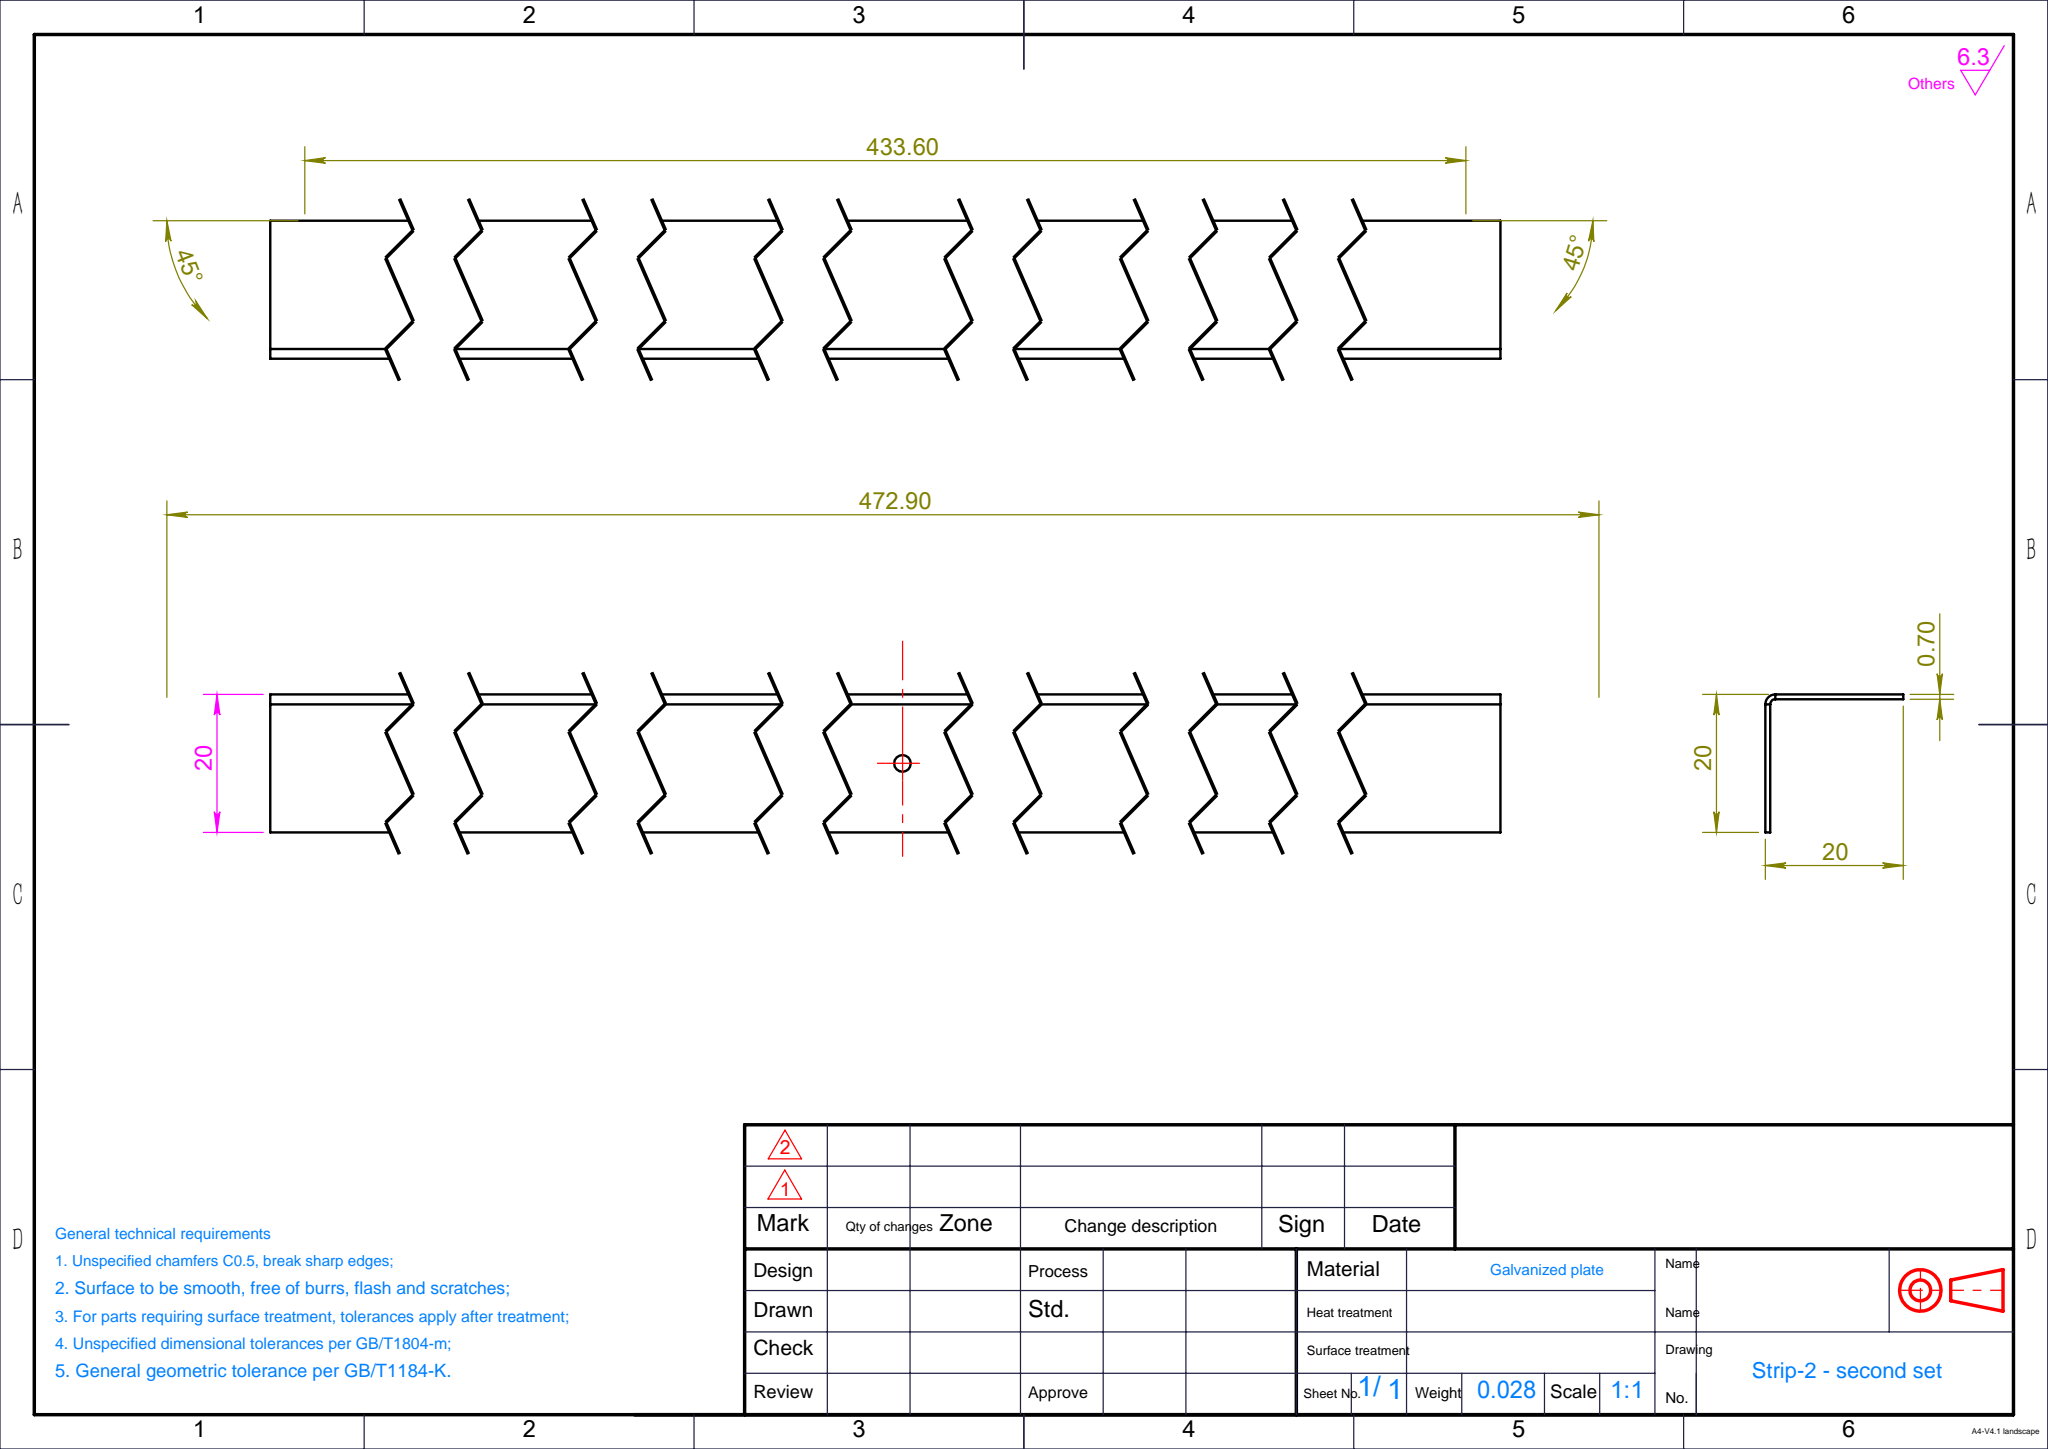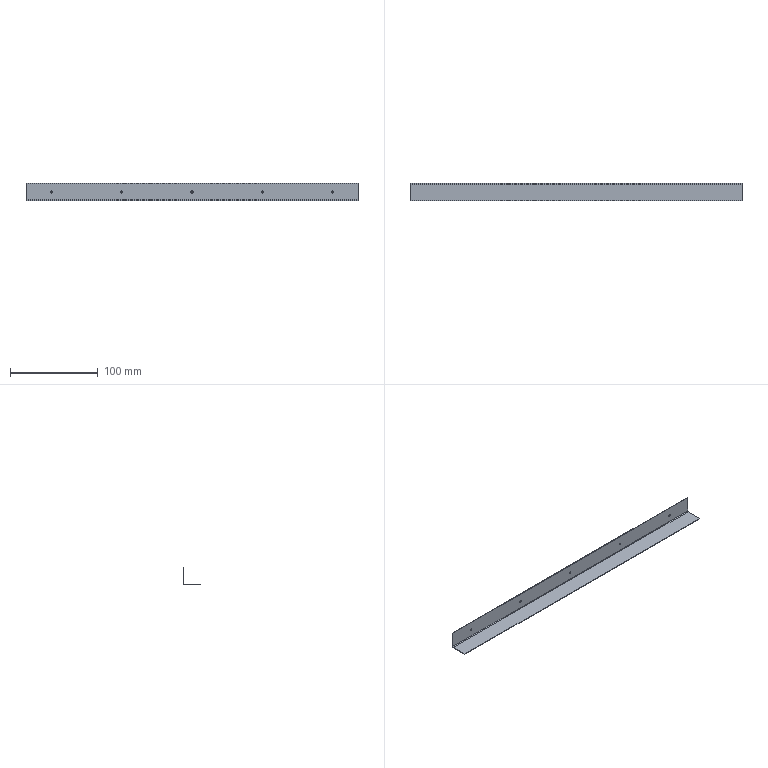Part | SolidWorks | features 3DProfileFeature 1, EdgeFlange 1, FlatPattern 1, HoleWzd 1, LPattern 1, MirrorPattern 1, SMBaseFlange 1, SheetMetal 1 | 1 solid | 24 faces | box 378 x 20 x 20 mm | volume 10260 mm3 | cylinder 12 | plane 12 | commonest cylinder face diameters 2.4 x10 1.473 x1 2.873 x1
STEP:
#1=CARTESIAN_POINT('',(-80.,9.3,10.5));
#2=VERTEX_POINT('',#1);
#3=CARTESIAN_POINT('',(-80.,9.3,8.1));
#4=VERTEX_POINT('',#3);
#5=CARTESIAN_POINT('',(-80.,9.3,9.3));
#6=DIRECTION('',(0.,-1.,0.));
#7=DIRECTION('',(0.,0.,1.));
#8=AXIS2_PLACEMENT_3D('',#5,#6,#7);
#9=CIRCLE('',#8,1.2);
#10=EDGE_CURVE('',#2,#4,#9,.T.);
#11=ORIENTED_EDGE('',*,*,#10,.T.);
#12=CARTESIAN_POINT('',(-80.,10.,8.1));
#13=VERTEX_POINT('',#12);
#14=CARTESIAN_POINT('',(-80.,10.,8.1));
#15=DIRECTION('',(0.,1.,0.));
#16=VECTOR('',#15,1000.);
#17=LINE('',#14,#16);
#18=EDGE_CURVE('',#4,#13,#17,.T.);
#19=ORIENTED_EDGE('',*,*,#18,.T.);
#20=CARTESIAN_POINT('',(-80.,10.,10.5));
#21=VERTEX_POINT('',#20);
#22=CARTESIAN_POINT('',(-80.,10.,9.3));
#23=DIRECTION('',(0.,-1.,0.));
#24=DIRECTION('',(0.,0.,1.));
#25=AXIS2_PLACEMENT_3D('',#22,#23,#24);
#26=CIRCLE('',#25,1.2);
#27=EDGE_CURVE('',#21,#13,#26,.T.);
#28=ORIENTED_EDGE('',*,*,#27,.F.);
#29=CARTESIAN_POINT('',(-80.,10.,10.5));
#30=DIRECTION('',(0.,1.,0.));
#31=VECTOR('',#30,1000.);
#32=LINE('',#29,#31);
#33=EDGE_CURVE('',#2,#21,#32,.T.);
#34=ORIENTED_EDGE('',*,*,#33,.F.);
#35=EDGE_LOOP('',(#11,#19,#28,#34));
#36=FACE_OUTER_BOUND('',#35,.T.);
#37=CARTESIAN_POINT('',(-80.,10.,9.3));
#38=DIRECTION('',(0.,1.,0.));
#39=DIRECTION('',(0.,0.,1.));
#40=AXIS2_PLACEMENT_3D('',#37,#38,#39);
#41=CYLINDRICAL_SURFACE('',#40,1.2);
#42=ADVANCED_FACE('',(#36),#41,.F.);
#43=CARTESIAN_POINT('',(-160.,9.3,10.5));
#44=VERTEX_POINT('',#43);
#45=CARTESIAN_POINT('',(-160.,9.3,8.1));
#46=VERTEX_POINT('',#45);
#47=CARTESIAN_POINT('',(-160.,9.3,9.3));
#48=DIRECTION('',(0.,-1.,0.));
#49=DIRECTION('',(0.,0.,1.));
#50=AXIS2_PLACEMENT_3D('',#47,#48,#49);
#51=CIRCLE('',#50,1.2);
#52=EDGE_CURVE('',#44,#46,#51,.T.);
#53=ORIENTED_EDGE('',*,*,#52,.T.);
#54=CARTESIAN_POINT('',(-160.,10.,8.1));
#55=VERTEX_POINT('',#54);
#56=CARTESIAN_POINT('',(-160.,10.,8.1));
#57=DIRECTION('',(0.,1.,0.));
#58=VECTOR('',#57,1000.);
#59=LINE('',#56,#58);
#60=EDGE_CURVE('',#46,#55,#59,.T.);
#61=ORIENTED_EDGE('',*,*,#60,.T.);
#62=CARTESIAN_POINT('',(-160.,10.,10.5));
#63=VERTEX_POINT('',#62);
#64=CARTESIAN_POINT('',(-160.,10.,9.3));
#65=DIRECTION('',(0.,-1.,0.));
#66=DIRECTION('',(0.,0.,1.));
#67=AXIS2_PLACEMENT_3D('',#64,#65,#66);
#68=CIRCLE('',#67,1.2);
#69=EDGE_CURVE('',#63,#55,#68,.T.);
#70=ORIENTED_EDGE('',*,*,#69,.F.);
#71=CARTESIAN_POINT('',(-160.,10.,10.5));
#72=DIRECTION('',(0.,1.,0.));
#73=VECTOR('',#72,1000.);
#74=LINE('',#71,#73);
#75=EDGE_CURVE('',#44,#63,#74,.T.);
#76=ORIENTED_EDGE('',*,*,#75,.F.);
#77=EDGE_LOOP('',(#53,#61,#70,#76));
#78=FACE_OUTER_BOUND('',#77,.T.);
#79=CARTESIAN_POINT('',(-160.,10.,9.3));
#80=DIRECTION('',(0.,1.,0.));
#81=DIRECTION('',(0.,0.,1.));
#82=AXIS2_PLACEMENT_3D('',#79,#80,#81);
#83=CYLINDRICAL_SURFACE('',#82,1.2);
#84=ADVANCED_FACE('',(#78),#83,.F.);
#85=CARTESIAN_POINT('',(160.,9.3,8.1));
#86=VERTEX_POINT('',#85);
#87=CARTESIAN_POINT('',(160.,9.3,10.5));
#88=VERTEX_POINT('',#87);
#89=CARTESIAN_POINT('',(160.,9.3,9.3));
#90=DIRECTION('',(0.,1.,0.));
#91=DIRECTION('',(0.,0.,1.));
#92=AXIS2_PLACEMENT_3D('',#89,#90,#91);
#93=CIRCLE('',#92,1.2);
#94=EDGE_CURVE('',#86,#88,#93,.T.);
#95=ORIENTED_EDGE('',*,*,#94,.F.);
#96=CARTESIAN_POINT('',(160.,10.,8.1));
#97=VERTEX_POINT('',#96);
#98=CARTESIAN_POINT('',(160.,10.,8.1));
#99=DIRECTION('',(0.,1.,0.));
#100=VECTOR('',#99,1000.);
#101=LINE('',#98,#100);
#102=EDGE_CURVE('',#86,#97,#101,.T.);
#103=ORIENTED_EDGE('',*,*,#102,.T.);
#104=CARTESIAN_POINT('',(160.,10.,10.5));
#105=VERTEX_POINT('',#104);
#106=CARTESIAN_POINT('',(160.,10.,9.3));
#107=DIRECTION('',(0.,1.,0.));
#108=DIRECTION('',(0.,0.,1.));
#109=AXIS2_PLACEMENT_3D('',#106,#107,#108);
#110=CIRCLE('',#109,1.2);
#111=EDGE_CURVE('',#97,#105,#110,.T.);
#112=ORIENTED_EDGE('',*,*,#111,.T.);
#113=CARTESIAN_POINT('',(160.,10.,10.5));
#114=DIRECTION('',(0.,1.,0.));
#115=VECTOR('',#114,1000.);
#116=LINE('',#113,#115);
#117=EDGE_CURVE('',#88,#105,#116,.T.);
#118=ORIENTED_EDGE('',*,*,#117,.F.);
#119=EDGE_LOOP('',(#95,#103,#112,#118));
#120=FACE_OUTER_BOUND('',#119,.T.);
#121=CARTESIAN_POINT('',(160.,10.,9.3));
#122=DIRECTION('',(0.,1.,0.));
#123=DIRECTION('',(0.,0.,1.));
#124=AXIS2_PLACEMENT_3D('',#121,#122,#123);
#125=CYLINDRICAL_SURFACE('',#124,1.2);
#126=ADVANCED_FACE('',(#120),#125,.F.);
#127=CARTESIAN_POINT('',(80.,9.3,8.1));
#128=VERTEX_POINT('',#127);
#129=CARTESIAN_POINT('',(80.,9.3,10.5));
#130=VERTEX_POINT('',#129);
#131=CARTESIAN_POINT('',(80.,9.3,9.3));
#132=DIRECTION('',(0.,1.,0.));
#133=DIRECTION('',(0.,0.,1.));
#134=AXIS2_PLACEMENT_3D('',#131,#132,#133);
#135=CIRCLE('',#134,1.2);
#136=EDGE_CURVE('',#128,#130,#135,.T.);
#137=ORIENTED_EDGE('',*,*,#136,.F.);
#138=CARTESIAN_POINT('',(80.,10.,8.1));
#139=VERTEX_POINT('',#138);
#140=CARTESIAN_POINT('',(80.,10.,8.1));
#141=DIRECTION('',(0.,1.,0.));
#142=VECTOR('',#141,1000.);
#143=LINE('',#140,#142);
#144=EDGE_CURVE('',#128,#139,#143,.T.);
#145=ORIENTED_EDGE('',*,*,#144,.T.);
#146=CARTESIAN_POINT('',(80.,10.,10.5));
#147=VERTEX_POINT('',#146);
#148=CARTESIAN_POINT('',(80.,10.,9.3));
#149=DIRECTION('',(0.,1.,0.));
#150=DIRECTION('',(0.,0.,1.));
#151=AXIS2_PLACEMENT_3D('',#148,#149,#150);
#152=CIRCLE('',#151,1.2);
#153=EDGE_CURVE('',#139,#147,#152,.T.);
#154=ORIENTED_EDGE('',*,*,#153,.T.);
#155=CARTESIAN_POINT('',(80.,10.,10.5));
#156=DIRECTION('',(0.,1.,0.));
#157=VECTOR('',#156,1000.);
#158=LINE('',#155,#157);
#159=EDGE_CURVE('',#130,#147,#158,.T.);
#160=ORIENTED_EDGE('',*,*,#159,.F.);
#161=EDGE_LOOP('',(#137,#145,#154,#160));
#162=FACE_OUTER_BOUND('',#161,.T.);
#163=CARTESIAN_POINT('',(80.,10.,9.3));
#164=DIRECTION('',(0.,1.,0.));
#165=DIRECTION('',(0.,0.,1.));
#166=AXIS2_PLACEMENT_3D('',#163,#164,#165);
#167=CYLINDRICAL_SURFACE('',#166,1.2);
#168=ADVANCED_FACE('',(#162),#167,.F.);
#169=CARTESIAN_POINT('',(0.,9.3,8.1));
#170=VERTEX_POINT('',#169);
#171=CARTESIAN_POINT('',(0.,9.3,10.5));
#172=VERTEX_POINT('',#171);
#173=CARTESIAN_POINT('',(0.,9.3,9.3));
#174=DIRECTION('',(0.,1.,0.));
#175=DIRECTION('',(0.,0.,1.));
#176=AXIS2_PLACEMENT_3D('',#173,#174,#175);
#177=CIRCLE('',#176,1.2);
#178=EDGE_CURVE('',#170,#172,#177,.T.);
#179=ORIENTED_EDGE('',*,*,#178,.F.);
#180=CARTESIAN_POINT('',(0.,10.,8.1));
#181=VERTEX_POINT('',#180);
#182=CARTESIAN_POINT('',(0.,10.,8.1));
#183=DIRECTION('',(0.,1.,0.));
#184=VECTOR('',#183,1000.);
#185=LINE('',#182,#184);
#186=EDGE_CURVE('',#170,#181,#185,.T.);
#187=ORIENTED_EDGE('',*,*,#186,.T.);
#188=CARTESIAN_POINT('',(0.,10.,10.5));
#189=VERTEX_POINT('',#188);
#190=CARTESIAN_POINT('',(0.,10.,9.3));
#191=DIRECTION('',(0.,1.,0.));
#192=DIRECTION('',(0.,0.,1.));
#193=AXIS2_PLACEMENT_3D('',#190,#191,#192);
#194=CIRCLE('',#193,1.2);
#195=EDGE_CURVE('',#181,#189,#194,.T.);
#196=ORIENTED_EDGE('',*,*,#195,.T.);
#197=CARTESIAN_POINT('',(0.,10.,10.5));
#198=DIRECTION('',(0.,1.,0.));
#199=VECTOR('',#198,1000.);
#200=LINE('',#197,#199);
#201=EDGE_CURVE('',#172,#189,#200,.T.);
#202=ORIENTED_EDGE('',*,*,#201,.F.);
#203=EDGE_LOOP('',(#179,#187,#196,#202));
#204=FACE_OUTER_BOUND('',#203,.T.);
#205=CARTESIAN_POINT('',(0.,10.,9.3));
#206=DIRECTION('',(0.,1.,0.));
#207=DIRECTION('',(0.,0.,1.));
#208=AXIS2_PLACEMENT_3D('',#205,#206,#207);
#209=CYLINDRICAL_SURFACE('',#208,1.2);
#210=ADVANCED_FACE('',(#204),#209,.F.);
#211=CARTESIAN_POINT('',(-189.,8.563,0.));
#212=VERTEX_POINT('',#211);
#213=CARTESIAN_POINT('',(-189.,-10.,0.));
#214=VERTEX_POINT('',#213);
#215=CARTESIAN_POINT('',(-189.,10.,0.));
#216=DIRECTION('',(0.,-1.,0.));
#217=VECTOR('',#216,1000.);
#218=LINE('',#215,#217);
#219=EDGE_CURVE('',#212,#214,#218,.T.);
#220=ORIENTED_EDGE('',*,*,#219,.F.);
#221=CARTESIAN_POINT('',(-189.,8.563,-0.7));
#222=VERTEX_POINT('',#221);
#223=CARTESIAN_POINT('',(-189.,8.563,0.));
#224=DIRECTION('',(0.,0.,-1.));
#225=VECTOR('',#224,1000.);
#226=LINE('',#223,#225);
#227=EDGE_CURVE('',#212,#222,#226,.T.);
#228=ORIENTED_EDGE('',*,*,#227,.T.);
#229=CARTESIAN_POINT('',(-189.,-10.,-0.7));
#230=VERTEX_POINT('',#229);
#231=CARTESIAN_POINT('',(-189.,10.,-0.7));
#232=DIRECTION('',(0.,-1.,0.));
#233=VECTOR('',#232,1000.);
#234=LINE('',#231,#233);
#235=EDGE_CURVE('',#222,#230,#234,.T.);
#236=ORIENTED_EDGE('',*,*,#235,.T.);
#237=CARTESIAN_POINT('',(-189.,-10.,-0.7));
#238=DIRECTION('',(0.,0.,1.));
#239=VECTOR('',#238,1000.);
#240=LINE('',#237,#239);
#241=EDGE_CURVE('',#230,#214,#240,.T.);
#242=ORIENTED_EDGE('',*,*,#241,.T.);
#243=EDGE_LOOP('',(#220,#228,#236,#242));
#244=FACE_OUTER_BOUND('',#243,.T.);
#245=CARTESIAN_POINT('',(-189.,10.,-0.7));
#246=DIRECTION('',(-1.,0.,0.));
#247=DIRECTION('',(0.,0.,1.));
#248=AXIS2_PLACEMENT_3D('',#245,#246,#247);
#249=PLANE('',#248);
#250=ADVANCED_FACE('',(#244),#249,.T.);
#251=CARTESIAN_POINT('',(189.,8.563,-0.7));
#252=VERTEX_POINT('',#251);
#253=CARTESIAN_POINT('',(-189.,8.563,-0.7));
#254=DIRECTION('',(1.,0.,0.));
#255=VECTOR('',#254,1000.);
#256=LINE('',#253,#255);
#257=EDGE_CURVE('',#222,#252,#256,.T.);
#258=ORIENTED_EDGE('',*,*,#257,.T.);
#259=CARTESIAN_POINT('',(189.,-10.,-0.7));
#260=VERTEX_POINT('',#259);
#261=CARTESIAN_POINT('',(189.,10.,-0.7));
#262=DIRECTION('',(0.,1.,0.));
#263=VECTOR('',#262,1000.);
#264=LINE('',#261,#263);
#265=EDGE_CURVE('',#260,#252,#264,.T.);
#266=ORIENTED_EDGE('',*,*,#265,.F.);
#267=CARTESIAN_POINT('',(-189.,-10.,-0.7));
#268=DIRECTION('',(1.,0.,0.));
#269=VECTOR('',#268,1000.);
#270=LINE('',#267,#269);
#271=EDGE_CURVE('',#230,#260,#270,.T.);
#272=ORIENTED_EDGE('',*,*,#271,.F.);
#273=ORIENTED_EDGE('',*,*,#235,.F.);
#274=EDGE_LOOP('',(#258,#266,#272,#273));
#275=FACE_OUTER_BOUND('',#274,.T.);
#276=CARTESIAN_POINT('',(0.,0.,-0.7));
#277=DIRECTION('',(0.,0.,1.));
#278=DIRECTION('',(1.,0.,0.));
#279=AXIS2_PLACEMENT_3D('',#276,#277,#278);
#280=PLANE('',#279);
#281=ADVANCED_FACE('',(#275),#280,.F.);
#282=CARTESIAN_POINT('',(189.,-10.,0.));
#283=VERTEX_POINT('',#282);
#284=CARTESIAN_POINT('',(189.,8.563,0.));
#285=VERTEX_POINT('',#284);
#286=CARTESIAN_POINT('',(189.,10.,0.));
#287=DIRECTION('',(0.,1.,0.));
#288=VECTOR('',#287,1000.);
#289=LINE('',#286,#288);
#290=EDGE_CURVE('',#283,#285,#289,.T.);
#291=ORIENTED_EDGE('',*,*,#290,.T.);
#292=CARTESIAN_POINT('',(-189.,8.563,0.));
#293=DIRECTION('',(1.,0.,0.));
#294=VECTOR('',#293,1000.);
#295=LINE('',#292,#294);
#296=EDGE_CURVE('',#212,#285,#295,.T.);
#297=ORIENTED_EDGE('',*,*,#296,.F.);
#298=ORIENTED_EDGE('',*,*,#219,.T.);
#299=CARTESIAN_POINT('',(-189.,-10.,0.));
#300=DIRECTION('',(1.,0.,0.));
#301=VECTOR('',#300,1000.);
#302=LINE('',#299,#301);
#303=EDGE_CURVE('',#214,#283,#302,.T.);
#304=ORIENTED_EDGE('',*,*,#303,.T.);
#305=EDGE_LOOP('',(#291,#297,#298,#304));
#306=FACE_OUTER_BOUND('',#305,.T.);
#307=CARTESIAN_POINT('',(0.,0.,0.));
#308=DIRECTION('',(0.,0.,1.));
#309=DIRECTION('',(1.,0.,0.));
#310=AXIS2_PLACEMENT_3D('',#307,#308,#309);
#311=PLANE('',#310);
#312=ADVANCED_FACE('',(#306),#311,.T.);
#313=CARTESIAN_POINT('',(189.,8.563,0.));
#314=DIRECTION('',(0.,0.,-1.));
#315=VECTOR('',#314,1000.);
#316=LINE('',#313,#315);
#317=EDGE_CURVE('',#285,#252,#316,.T.);
#318=ORIENTED_EDGE('',*,*,#317,.F.);
#319=ORIENTED_EDGE('',*,*,#290,.F.);
#320=CARTESIAN_POINT('',(189.,-10.,-0.7));
#321=DIRECTION('',(0.,0.,1.));
#322=VECTOR('',#321,1000.);
#323=LINE('',#320,#322);
#324=EDGE_CURVE('',#260,#283,#323,.T.);
#325=ORIENTED_EDGE('',*,*,#324,.F.);
#326=ORIENTED_EDGE('',*,*,#265,.T.);
#327=EDGE_LOOP('',(#318,#319,#325,#326));
#328=FACE_OUTER_BOUND('',#327,.T.);
#329=CARTESIAN_POINT('',(189.,10.,-0.7));
#330=DIRECTION('',(1.,0.,0.));
#331=DIRECTION('',(0.,0.,-1.));
#332=AXIS2_PLACEMENT_3D('',#329,#330,#331);
#333=PLANE('',#332);
#334=ADVANCED_FACE('',(#328),#333,.T.);
#335=ORIENTED_EDGE('',*,*,#303,.F.);
#336=ORIENTED_EDGE('',*,*,#241,.F.);
#337=ORIENTED_EDGE('',*,*,#271,.T.);
#338=ORIENTED_EDGE('',*,*,#324,.T.);
#339=EDGE_LOOP('',(#335,#336,#337,#338));
#340=FACE_OUTER_BOUND('',#339,.T.);
#341=CARTESIAN_POINT('',(-189.,-10.,-0.7));
#342=DIRECTION('',(0.,-1.,0.));
#343=DIRECTION('',(0.,0.,-1.));
#344=AXIS2_PLACEMENT_3D('',#341,#342,#343);
#345=PLANE('',#344);
#346=ADVANCED_FACE('',(#340),#345,.T.);
#347=CARTESIAN_POINT('',(189.,9.3,0.7366));
#348=VERTEX_POINT('',#347);
#349=CARTESIAN_POINT('',(189.,10.,0.7366));
#350=VERTEX_POINT('',#349);
#351=CARTESIAN_POINT('',(189.,10.,0.7366));
#352=DIRECTION('',(0.,1.,0.));
#353=VECTOR('',#352,1000.);
#354=LINE('',#351,#353);
#355=EDGE_CURVE('',#348,#350,#354,.T.);
#356=ORIENTED_EDGE('',*,*,#355,.F.);
#357=CARTESIAN_POINT('',(189.,8.563,0.7366));
#358=DIRECTION('',(1.,0.,0.));
#359=DIRECTION('',(0.,0.,1.));
#360=AXIS2_PLACEMENT_3D('',#357,#358,#359);
#361=CIRCLE('',#360,0.7366);
#362=EDGE_CURVE('',#285,#348,#361,.T.);
#363=ORIENTED_EDGE('',*,*,#362,.F.);
#364=ORIENTED_EDGE('',*,*,#317,.T.);
#365=CARTESIAN_POINT('',(189.,8.563,0.7366));
#366=DIRECTION('',(1.,0.,0.));
#367=DIRECTION('',(0.,0.,1.));
#368=AXIS2_PLACEMENT_3D('',#365,#366,#367);
#369=CIRCLE('',#368,1.437);
#370=EDGE_CURVE('',#252,#350,#369,.T.);
#371=ORIENTED_EDGE('',*,*,#370,.T.);
#372=EDGE_LOOP('',(#356,#363,#364,#371));
#373=FACE_OUTER_BOUND('',#372,.T.);
#374=CARTESIAN_POINT('',(189.,8.563,0.7366));
#375=DIRECTION('',(1.,0.,0.));
#376=DIRECTION('',(0.,0.,-1.));
#377=AXIS2_PLACEMENT_3D('',#374,#375,#376);
#378=PLANE('',#377);
#379=ADVANCED_FACE('',(#373),#378,.T.);
#380=CARTESIAN_POINT('',(-189.,9.3,0.7366));
#381=VERTEX_POINT('',#380);
#382=CARTESIAN_POINT('',(-189.,8.563,0.7366));
#383=DIRECTION('',(-1.,0.,0.));
#384=DIRECTION('',(0.,0.,1.));
#385=AXIS2_PLACEMENT_3D('',#382,#383,#384);
#386=CIRCLE('',#385,0.7366);
#387=EDGE_CURVE('',#381,#212,#386,.T.);
#388=ORIENTED_EDGE('',*,*,#387,.F.);
#389=CARTESIAN_POINT('',(-189.,10.,0.7366));
#390=VERTEX_POINT('',#389);
#391=CARTESIAN_POINT('',(-189.,9.3,0.7366));
#392=DIRECTION('',(0.,1.,0.));
#393=VECTOR('',#392,1000.);
#394=LINE('',#391,#393);
#395=EDGE_CURVE('',#381,#390,#394,.T.);
#396=ORIENTED_EDGE('',*,*,#395,.T.);
#397=CARTESIAN_POINT('',(-189.,8.563,0.7366));
#398=DIRECTION('',(-1.,0.,0.));
#399=DIRECTION('',(0.,0.,1.));
#400=AXIS2_PLACEMENT_3D('',#397,#398,#399);
#401=CIRCLE('',#400,1.437);
#402=EDGE_CURVE('',#390,#222,#401,.T.);
#403=ORIENTED_EDGE('',*,*,#402,.T.);
#404=ORIENTED_EDGE('',*,*,#227,.F.);
#405=EDGE_LOOP('',(#388,#396,#403,#404));
#406=FACE_OUTER_BOUND('',#405,.T.);
#407=CARTESIAN_POINT('',(-189.,8.563,0.7366));
#408=DIRECTION('',(1.,0.,0.));
#409=DIRECTION('',(0.,0.,-1.));
#410=AXIS2_PLACEMENT_3D('',#407,#408,#409);
#411=PLANE('',#410);
#412=ADVANCED_FACE('',(#406),#411,.F.);
#413=ORIENTED_EDGE('',*,*,#257,.F.);
#414=ORIENTED_EDGE('',*,*,#402,.F.);
#415=CARTESIAN_POINT('',(0.,10.,0.7366));
#416=DIRECTION('',(-1.,0.,0.));
#417=VECTOR('',#416,1000.);
#418=LINE('',#415,#417);
#419=EDGE_CURVE('',#350,#390,#418,.T.);
#420=ORIENTED_EDGE('',*,*,#419,.F.);
#421=ORIENTED_EDGE('',*,*,#370,.F.);
#422=EDGE_LOOP('',(#413,#414,#420,#421));
#423=FACE_OUTER_BOUND('',#422,.T.);
#424=CARTESIAN_POINT('',(-189.,8.563,0.7366));
#425=DIRECTION('',(-1.,0.,0.));
#426=DIRECTION('',(0.,1.,0.));
#427=AXIS2_PLACEMENT_3D('',#424,#425,#426);
#428=CYLINDRICAL_SURFACE('',#427,1.437);
#429=ADVANCED_FACE('',(#423),#428,.T.);
#430=ORIENTED_EDGE('',*,*,#296,.T.);
#431=ORIENTED_EDGE('',*,*,#362,.T.);
#432=CARTESIAN_POINT('',(189.,9.3,0.7366));
#433=DIRECTION('',(-1.,0.,0.));
#434=VECTOR('',#433,1000.);
#435=LINE('',#432,#434);
#436=EDGE_CURVE('',#348,#381,#435,.T.);
#437=ORIENTED_EDGE('',*,*,#436,.T.);
#438=ORIENTED_EDGE('',*,*,#387,.T.);
#439=EDGE_LOOP('',(#430,#431,#437,#438));
#440=FACE_OUTER_BOUND('',#439,.T.);
#441=CARTESIAN_POINT('',(-189.,8.563,0.7366));
#442=DIRECTION('',(-1.,0.,0.));
#443=DIRECTION('',(0.,1.,0.));
#444=AXIS2_PLACEMENT_3D('',#441,#442,#443);
#445=CYLINDRICAL_SURFACE('',#444,0.7366);
#446=ADVANCED_FACE('',(#440),#445,.F.);
#447=CARTESIAN_POINT('',(-189.,10.,19.3));
#448=VERTEX_POINT('',#447);
#449=CARTESIAN_POINT('',(-189.,10.,0.));
#450=DIRECTION('',(0.,0.,-1.));
#451=VECTOR('',#450,1000.);
#452=LINE('',#449,#451);
#453=EDGE_CURVE('',#448,#390,#452,.T.);
#454=ORIENTED_EDGE('',*,*,#453,.T.);
#455=ORIENTED_EDGE('',*,*,#395,.F.);
#456=CARTESIAN_POINT('',(-189.,9.3,19.3));
#457=VERTEX_POINT('',#456);
#458=CARTESIAN_POINT('',(-189.,9.3,0.));
#459=DIRECTION('',(0.,0.,-1.));
#460=VECTOR('',#459,1000.);
#461=LINE('',#458,#460);
#462=EDGE_CURVE('',#457,#381,#461,.T.);
#463=ORIENTED_EDGE('',*,*,#462,.F.);
#464=CARTESIAN_POINT('',(-189.,10.,19.3));
#465=DIRECTION('',(0.,-1.,0.));
#466=VECTOR('',#465,1000.);
#467=LINE('',#464,#466);
#468=EDGE_CURVE('',#448,#457,#467,.T.);
#469=ORIENTED_EDGE('',*,*,#468,.F.);
#470=EDGE_LOOP('',(#454,#455,#463,#469));
#471=FACE_OUTER_BOUND('',#470,.T.);
#472=CARTESIAN_POINT('',(-189.,10.,0.));
#473=DIRECTION('',(-1.,0.,0.));
#474=DIRECTION('',(0.,0.,1.));
#475=AXIS2_PLACEMENT_3D('',#472,#473,#474);
#476=PLANE('',#475);
#477=ADVANCED_FACE('',(#471),#476,.T.);
#478=CARTESIAN_POINT('',(189.,9.3,19.3));
#479=VERTEX_POINT('',#478);
#480=CARTESIAN_POINT('',(189.,9.3,0.));
#481=DIRECTION('',(0.,0.,1.));
#482=VECTOR('',#481,1000.);
#483=LINE('',#480,#482);
#484=EDGE_CURVE('',#348,#479,#483,.T.);
#485=ORIENTED_EDGE('',*,*,#484,.F.);
#486=ORIENTED_EDGE('',*,*,#355,.T.);
#487=CARTESIAN_POINT('',(189.,10.,19.3));
#488=VERTEX_POINT('',#487);
#489=CARTESIAN_POINT('',(189.,10.,19.3));
#490=DIRECTION('',(0.,0.,1.));
#491=VECTOR('',#490,1000.);
#492=LINE('',#489,#491);
#493=EDGE_CURVE('',#350,#488,#492,.T.);
#494=ORIENTED_EDGE('',*,*,#493,.T.);
#495=CARTESIAN_POINT('',(189.,10.,19.3));
#496=DIRECTION('',(0.,-1.,0.));
#497=VECTOR('',#496,1000.);
#498=LINE('',#495,#497);
#499=EDGE_CURVE('',#488,#479,#498,.T.);
#500=ORIENTED_EDGE('',*,*,#499,.T.);
#501=EDGE_LOOP('',(#485,#486,#494,#500));
#502=FACE_OUTER_BOUND('',#501,.T.);
#503=CARTESIAN_POINT('',(189.,10.,19.3));
#504=DIRECTION('',(1.,0.,0.));
#505=DIRECTION('',(0.,0.,-1.));
#506=AXIS2_PLACEMENT_3D('',#503,#504,#505);
#507=PLANE('',#506);
#508=ADVANCED_FACE('',(#502),#507,.T.);
#509=ORIENTED_EDGE('',*,*,#27,.T.);
#510=CARTESIAN_POINT('',(-80.,10.,9.3));
#511=DIRECTION('',(0.,-1.,0.));
#512=DIRECTION('',(0.,0.,1.));
#513=AXIS2_PLACEMENT_3D('',#510,#511,#512);
#514=CIRCLE('',#513,1.2);
#515=EDGE_CURVE('',#13,#21,#514,.T.);
#516=ORIENTED_EDGE('',*,*,#515,.T.);
#517=EDGE_LOOP('',(#509,#516));
#518=FACE_BOUND('',#517,.T.);
#519=ORIENTED_EDGE('',*,*,#69,.T.);
#520=CARTESIAN_POINT('',(-160.,10.,9.3));
#521=DIRECTION('',(0.,-1.,0.));
#522=DIRECTION('',(0.,0.,1.));
#523=AXIS2_PLACEMENT_3D('',#520,#521,#522);
#524=CIRCLE('',#523,1.2);
#525=EDGE_CURVE('',#55,#63,#524,.T.);
#526=ORIENTED_EDGE('',*,*,#525,.T.);
#527=EDGE_LOOP('',(#519,#526));
#528=FACE_BOUND('',#527,.T.);
#529=CARTESIAN_POINT('',(160.,10.,9.3));
#530=DIRECTION('',(0.,1.,0.));
#531=DIRECTION('',(0.,0.,1.));
#532=AXIS2_PLACEMENT_3D('',#529,#530,#531);
#533=CIRCLE('',#532,1.2);
#534=EDGE_CURVE('',#105,#97,#533,.T.);
#535=ORIENTED_EDGE('',*,*,#534,.F.);
#536=ORIENTED_EDGE('',*,*,#111,.F.);
#537=EDGE_LOOP('',(#535,#536));
#538=FACE_BOUND('',#537,.T.);
#539=CARTESIAN_POINT('',(80.,10.,9.3));
#540=DIRECTION('',(0.,1.,0.));
#541=DIRECTION('',(0.,0.,1.));
#542=AXIS2_PLACEMENT_3D('',#539,#540,#541);
#543=CIRCLE('',#542,1.2);
#544=EDGE_CURVE('',#147,#139,#543,.T.);
#545=ORIENTED_EDGE('',*,*,#544,.F.);
#546=ORIENTED_EDGE('',*,*,#153,.F.);
#547=EDGE_LOOP('',(#545,#546));
#548=FACE_BOUND('',#547,.T.);
#549=CARTESIAN_POINT('',(0.,10.,9.3));
#550=DIRECTION('',(0.,1.,0.));
#551=DIRECTION('',(0.,0.,1.));
#552=AXIS2_PLACEMENT_3D('',#549,#550,#551);
#553=CIRCLE('',#552,1.2);
#554=EDGE_CURVE('',#189,#181,#553,.T.);
#555=ORIENTED_EDGE('',*,*,#554,.F.);
#556=ORIENTED_EDGE('',*,*,#195,.F.);
#557=EDGE_LOOP('',(#555,#556));
#558=FACE_BOUND('',#557,.T.);
#559=ORIENTED_EDGE('',*,*,#493,.F.);
#560=ORIENTED_EDGE('',*,*,#419,.T.);
#561=ORIENTED_EDGE('',*,*,#453,.F.);
#562=CARTESIAN_POINT('',(-189.,10.,19.3));
#563=DIRECTION('',(-1.,0.,0.));
#564=VECTOR('',#563,1000.);
#565=LINE('',#562,#564);
#566=EDGE_CURVE('',#488,#448,#565,.T.);
#567=ORIENTED_EDGE('',*,*,#566,.F.);
#568=EDGE_LOOP('',(#559,#560,#561,#567));
#569=FACE_OUTER_BOUND('',#568,.T.);
#570=CARTESIAN_POINT('',(0.,10.,0.));
#571=DIRECTION('',(0.,1.,0.));
#572=DIRECTION('',(0.,0.,1.));
#573=AXIS2_PLACEMENT_3D('',#570,#571,#572);
#574=PLANE('',#573);
#575=ADVANCED_FACE('',(#518,#528,#538,#548,#558,#569),#574,.T.);
#576=ORIENTED_EDGE('',*,*,#10,.F.);
#577=CARTESIAN_POINT('',(-80.,9.3,9.3));
#578=DIRECTION('',(0.,-1.,0.));
#579=DIRECTION('',(0.,0.,1.));
#580=AXIS2_PLACEMENT_3D('',#577,#578,#579);
#581=CIRCLE('',#580,1.2);
#582=EDGE_CURVE('',#4,#2,#581,.T.);
#583=ORIENTED_EDGE('',*,*,#582,.F.);
#584=EDGE_LOOP('',(#576,#583));
#585=FACE_BOUND('',#584,.T.);
#586=ORIENTED_EDGE('',*,*,#52,.F.);
#587=CARTESIAN_POINT('',(-160.,9.3,9.3));
#588=DIRECTION('',(0.,-1.,0.));
#589=DIRECTION('',(0.,0.,1.));
#590=AXIS2_PLACEMENT_3D('',#587,#588,#589);
#591=CIRCLE('',#590,1.2);
#592=EDGE_CURVE('',#46,#44,#591,.T.);
#593=ORIENTED_EDGE('',*,*,#592,.F.);
#594=EDGE_LOOP('',(#586,#593));
#595=FACE_BOUND('',#594,.T.);
#596=CARTESIAN_POINT('',(160.,9.3,9.3));
#597=DIRECTION('',(0.,1.,0.));
#598=DIRECTION('',(0.,0.,1.));
#599=AXIS2_PLACEMENT_3D('',#596,#597,#598);
#600=CIRCLE('',#599,1.2);
#601=EDGE_CURVE('',#88,#86,#600,.T.);
#602=ORIENTED_EDGE('',*,*,#601,.T.);
#603=ORIENTED_EDGE('',*,*,#94,.T.);
#604=EDGE_LOOP('',(#602,#603));
#605=FACE_BOUND('',#604,.T.);
#606=CARTESIAN_POINT('',(80.,9.3,9.3));
#607=DIRECTION('',(0.,1.,0.));
#608=DIRECTION('',(0.,0.,1.));
#609=AXIS2_PLACEMENT_3D('',#606,#607,#608);
#610=CIRCLE('',#609,1.2);
#611=EDGE_CURVE('',#130,#128,#610,.T.);
#612=ORIENTED_EDGE('',*,*,#611,.T.);
#613=ORIENTED_EDGE('',*,*,#136,.T.);
#614=EDGE_LOOP('',(#612,#613));
#615=FACE_BOUND('',#614,.T.);
#616=CARTESIAN_POINT('',(0.,9.3,9.3));
#617=DIRECTION('',(0.,1.,0.));
#618=DIRECTION('',(0.,0.,1.));
#619=AXIS2_PLACEMENT_3D('',#616,#617,#618);
#620=CIRCLE('',#619,1.2);
#621=EDGE_CURVE('',#172,#170,#620,.T.);
#622=ORIENTED_EDGE('',*,*,#621,.T.);
#623=ORIENTED_EDGE('',*,*,#178,.T.);
#624=EDGE_LOOP('',(#622,#623));
#625=FACE_BOUND('',#624,.T.);
#626=ORIENTED_EDGE('',*,*,#436,.F.);
#627=ORIENTED_EDGE('',*,*,#484,.T.);
#628=CARTESIAN_POINT('',(0.,9.3,19.3));
#629=DIRECTION('',(-1.,0.,0.));
#630=VECTOR('',#629,1000.);
#631=LINE('',#628,#630);
#632=EDGE_CURVE('',#479,#457,#631,.T.);
#633=ORIENTED_EDGE('',*,*,#632,.T.);
#634=ORIENTED_EDGE('',*,*,#462,.T.);
#635=EDGE_LOOP('',(#626,#627,#633,#634));
#636=FACE_OUTER_BOUND('',#635,.T.);
#637=CARTESIAN_POINT('',(0.,9.3,0.));
#638=DIRECTION('',(0.,1.,0.));
#639=DIRECTION('',(0.,0.,1.));
#640=AXIS2_PLACEMENT_3D('',#637,#638,#639);
#641=PLANE('',#640);
#642=ADVANCED_FACE('',(#585,#595,#605,#615,#625,#636),#641,.F.);
#643=ORIENTED_EDGE('',*,*,#632,.F.);
#644=ORIENTED_EDGE('',*,*,#499,.F.);
#645=ORIENTED_EDGE('',*,*,#566,.T.);
#646=ORIENTED_EDGE('',*,*,#468,.T.);
#647=EDGE_LOOP('',(#643,#644,#645,#646));
#648=FACE_OUTER_BOUND('',#647,.T.);
#649=CARTESIAN_POINT('',(-189.,10.,19.3));
#650=DIRECTION('',(0.,0.,1.));
#651=DIRECTION('',(0.,-1.,0.));
#652=AXIS2_PLACEMENT_3D('',#649,#650,#651);
#653=PLANE('',#652);
#654=ADVANCED_FACE('',(#648),#653,.T.);
#655=ORIENTED_EDGE('',*,*,#186,.F.);
#656=ORIENTED_EDGE('',*,*,#621,.F.);
#657=ORIENTED_EDGE('',*,*,#201,.T.);
#658=ORIENTED_EDGE('',*,*,#554,.T.);
#659=EDGE_LOOP('',(#655,#656,#657,#658));
#660=FACE_OUTER_BOUND('',#659,.T.);
#661=CARTESIAN_POINT('',(0.,10.,9.3));
#662=DIRECTION('',(0.,1.,0.));
#663=DIRECTION('',(0.,0.,1.));
#664=AXIS2_PLACEMENT_3D('',#661,#662,#663);
#665=CYLINDRICAL_SURFACE('',#664,1.2);
#666=ADVANCED_FACE('',(#660),#665,.F.);
#667=ORIENTED_EDGE('',*,*,#144,.F.);
#668=ORIENTED_EDGE('',*,*,#611,.F.);
#669=ORIENTED_EDGE('',*,*,#159,.T.);
#670=ORIENTED_EDGE('',*,*,#544,.T.);
#671=EDGE_LOOP('',(#667,#668,#669,#670));
#672=FACE_OUTER_BOUND('',#671,.T.);
#673=CARTESIAN_POINT('',(80.,10.,9.3));
#674=DIRECTION('',(0.,1.,0.));
#675=DIRECTION('',(0.,0.,1.));
#676=AXIS2_PLACEMENT_3D('',#673,#674,#675);
#677=CYLINDRICAL_SURFACE('',#676,1.2);
#678=ADVANCED_FACE('',(#672),#677,.F.);
#679=ORIENTED_EDGE('',*,*,#102,.F.);
#680=ORIENTED_EDGE('',*,*,#601,.F.);
#681=ORIENTED_EDGE('',*,*,#117,.T.);
#682=ORIENTED_EDGE('',*,*,#534,.T.);
#683=EDGE_LOOP('',(#679,#680,#681,#682));
#684=FACE_OUTER_BOUND('',#683,.T.);
#685=CARTESIAN_POINT('',(160.,10.,9.3));
#686=DIRECTION('',(0.,1.,0.));
#687=DIRECTION('',(0.,0.,1.));
#688=AXIS2_PLACEMENT_3D('',#685,#686,#687);
#689=CYLINDRICAL_SURFACE('',#688,1.2);
#690=ADVANCED_FACE('',(#684),#689,.F.);
#691=ORIENTED_EDGE('',*,*,#60,.F.);
#692=ORIENTED_EDGE('',*,*,#592,.T.);
#693=ORIENTED_EDGE('',*,*,#75,.T.);
#694=ORIENTED_EDGE('',*,*,#525,.F.);
#695=EDGE_LOOP('',(#691,#692,#693,#694));
#696=FACE_OUTER_BOUND('',#695,.T.);
#697=CARTESIAN_POINT('',(-160.,10.,9.3));
#698=DIRECTION('',(0.,1.,0.));
#699=DIRECTION('',(0.,0.,1.));
#700=AXIS2_PLACEMENT_3D('',#697,#698,#699);
#701=CYLINDRICAL_SURFACE('',#700,1.2);
#702=ADVANCED_FACE('',(#696),#701,.F.);
#703=ORIENTED_EDGE('',*,*,#18,.F.);
#704=ORIENTED_EDGE('',*,*,#582,.T.);
#705=ORIENTED_EDGE('',*,*,#33,.T.);
#706=ORIENTED_EDGE('',*,*,#515,.F.);
#707=EDGE_LOOP('',(#703,#704,#705,#706));
#708=FACE_OUTER_BOUND('',#707,.T.);
#709=CARTESIAN_POINT('',(-80.,10.,9.3));
#710=DIRECTION('',(0.,1.,0.));
#711=DIRECTION('',(0.,0.,1.));
#712=AXIS2_PLACEMENT_3D('',#709,#710,#711);
#713=CYLINDRICAL_SURFACE('',#712,1.2);
#714=ADVANCED_FACE('',(#708),#713,.F.);
#715=CLOSED_SHELL('',(#42,#84,#126,#168,#210,#250,#281,#312,#334,#346,#379,#412,#429,#446,#477,#508,#575,#642,#654,#666,#678,#690,#702,#714));
#716=MANIFOLD_SOLID_BREP('',#715);
#717=CARTESIAN_POINT('',(0.,0.,0.));
#718=DIRECTION('',(0.,0.,1.));
#719=DIRECTION('',(1.,0.,0.));
#720=AXIS2_PLACEMENT_3D('',#717,#718,#719);
#721=(LENGTH_UNIT()NAMED_UNIT(*)SI_UNIT(.MILLI.,.METRE.));
#722=UNCERTAINTY_MEASURE_WITH_UNIT(LENGTH_MEASURE(0.00001),#721,'','');
#723=(NAMED_UNIT(*)PLANE_ANGLE_UNIT()SI_UNIT($,.RADIAN.));
#724=(NAMED_UNIT(*)SI_UNIT($,.STERADIAN.)SOLID_ANGLE_UNIT());
#725=(GEOMETRIC_REPRESENTATION_CONTEXT(3)GLOBAL_UNCERTAINTY_ASSIGNED_CONTEXT((#722))GLOBAL_UNIT_ASSIGNED_CONTEXT((#721,#723,#724))REPRESENTATION_CONTEXT('',''));
#726=ADVANCED_BREP_SHAPE_REPRESENTATION('',(#716,#720),#725);